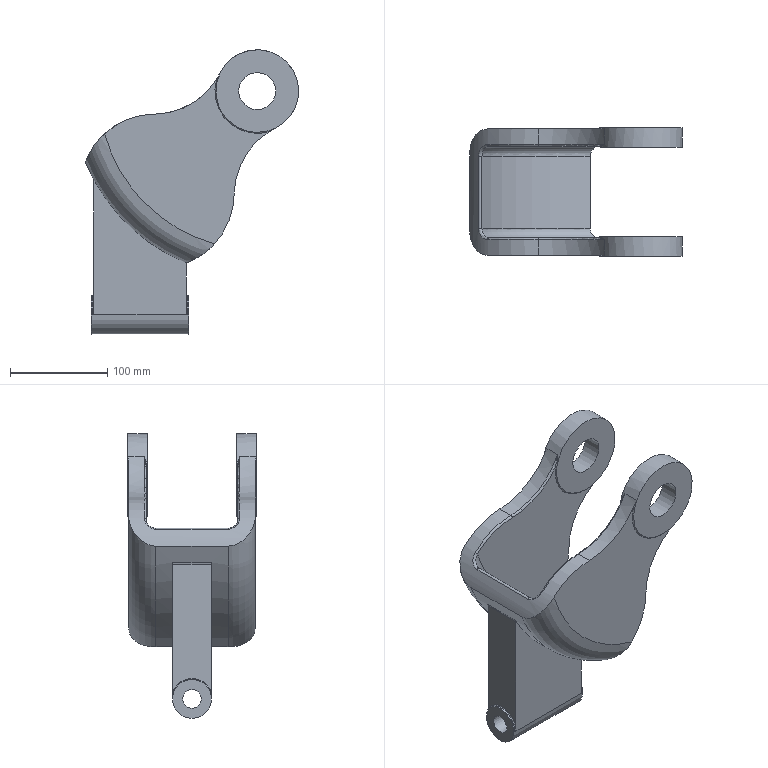Part | NX | features DATUM_CSYS 8, BLEND 7, EXTRUDE 7, SKETCH 7, EXTRACT_FACE 4, CPROJ 2, EXTRACT_DATUM_AXIS 2, EXTRACT_DATUM_PLANE 2, HOLE PACKAGE 2, Instance Feature 2, Mirror Feature 2, SIMPLE HOLE 2, DATUM_PLANE 1 | 1 solid | 49 faces | box 219.007 x 132 x 292.5 mm | volume 1450063 mm3 | cylinder 17 | plane 14 | torus 14 | spline 4 | commonest cylinder face diameters 152 x6 38 x2 85 x2 4 x1 5.7 x1 10 x1